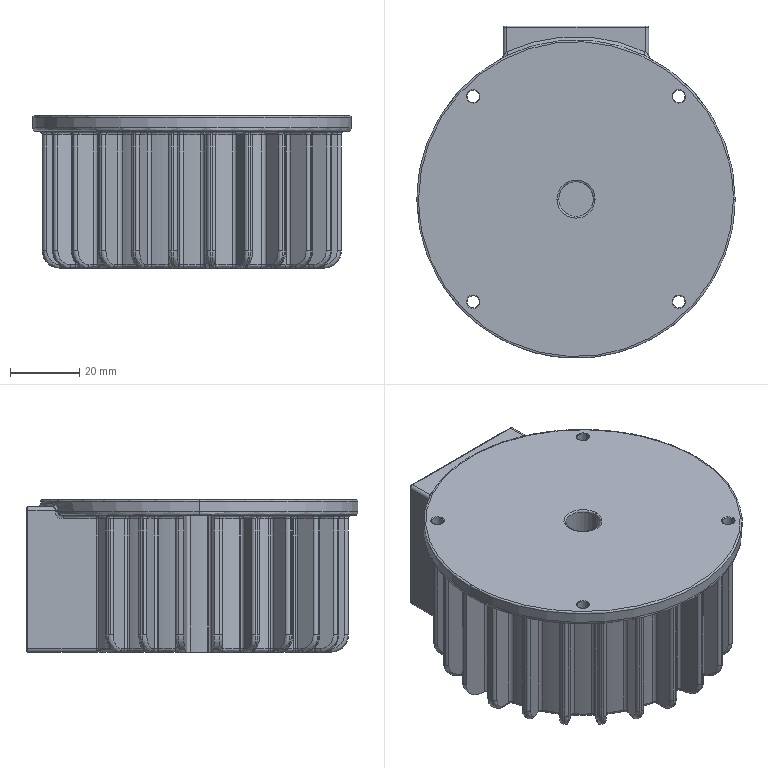Part | STEP file | 31090131--1-SOLI00 | 1 solid | 527 faces | box 92 x 96 x 44 mm | volume 202993 mm3 | cylinder 236 | spline 228 | plane 63 | commonest cylinder face diameters 2 x180 10 x20 72 x20 3.5 x8 1 x4 34 x2